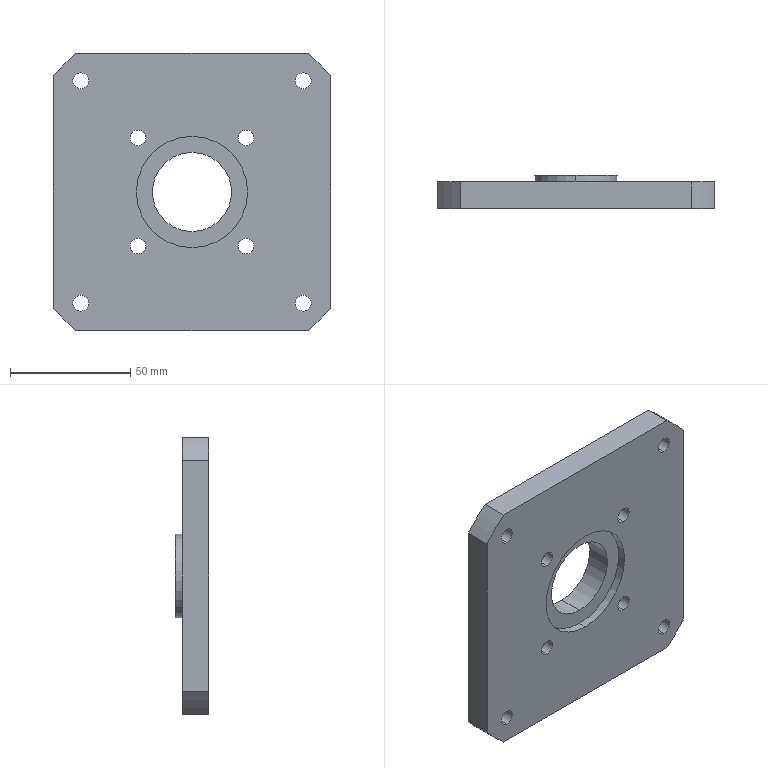Part | SolidWorks | features BaseBody 1 | 1 solid | 46 faces | box 115.385 x 13.846 x 115.385 mm | volume 127241 mm3 | cylinder 34 | plane 12 | commonest cylinder face diameters 6.577 x16 11.538 x8 150 x4 32.885 x2 34.615 x2 46.154 x2
STEP:
#1=CARTESIAN_POINT('',(184.809,206.,262.822));
#2=VERTEX_POINT('',#1);
#3=CARTESIAN_POINT('',(184.809,206.,274.36));
#4=VERTEX_POINT('',#3);
#5=CARTESIAN_POINT('',(184.809,206.,268.591));
#6=DIRECTION('',(0.,1.,0.));
#7=DIRECTION('',(0.,0.,1.));
#8=AXIS2_PLACEMENT_3D('',#5,#6,#7);
#9=CIRCLE('',#8,5.769);
#10=EDGE_CURVE('',#2,#4,#9,.T.);
#11=ORIENTED_EDGE('',*,*,#10,.F.);
#12=CARTESIAN_POINT('',(184.809,212.577,262.822));
#13=VERTEX_POINT('',#12);
#14=CARTESIAN_POINT('',(184.809,201.615,262.822));
#15=DIRECTION('',(0.,1.,0.));
#16=VECTOR('',#15,1000.);
#17=LINE('',#14,#16);
#18=EDGE_CURVE('',#2,#13,#17,.T.);
#19=ORIENTED_EDGE('',*,*,#18,.T.);
#20=CARTESIAN_POINT('',(184.809,212.577,274.36));
#21=VERTEX_POINT('',#20);
#22=CARTESIAN_POINT('',(184.809,212.577,268.591));
#23=DIRECTION('',(0.,1.,0.));
#24=DIRECTION('',(0.,0.,1.));
#25=AXIS2_PLACEMENT_3D('',#22,#23,#24);
#26=CIRCLE('',#25,5.769);
#27=EDGE_CURVE('',#13,#21,#26,.T.);
#28=ORIENTED_EDGE('',*,*,#27,.T.);
#29=CARTESIAN_POINT('',(184.809,201.615,274.36));
#30=DIRECTION('',(0.,1.,0.));
#31=VECTOR('',#30,1000.);
#32=LINE('',#29,#31);
#33=EDGE_CURVE('',#4,#21,#32,.T.);
#34=ORIENTED_EDGE('',*,*,#33,.F.);
#35=EDGE_LOOP('',(#11,#19,#28,#34));
#36=FACE_OUTER_BOUND('',#35,.T.);
#37=CARTESIAN_POINT('',(184.809,201.615,268.591));
#38=DIRECTION('',(0.,1.,0.));
#39=DIRECTION('',(0.,0.,1.));
#40=AXIS2_PLACEMENT_3D('',#37,#38,#39);
#41=CYLINDRICAL_SURFACE('',#40,5.769);
#42=ADVANCED_FACE('',(#36),#41,.F.);
#43=CARTESIAN_POINT('',(184.809,206.,217.948));
#44=VERTEX_POINT('',#43);
#45=CARTESIAN_POINT('',(184.809,206.,229.486));
#46=VERTEX_POINT('',#45);
#47=CARTESIAN_POINT('',(184.809,206.,223.717));
#48=DIRECTION('',(0.,1.,0.));
#49=DIRECTION('',(0.,0.,1.));
#50=AXIS2_PLACEMENT_3D('',#47,#48,#49);
#51=CIRCLE('',#50,5.769);
#52=EDGE_CURVE('',#44,#46,#51,.T.);
#53=ORIENTED_EDGE('',*,*,#52,.F.);
#54=CARTESIAN_POINT('',(184.809,212.577,217.948));
#55=VERTEX_POINT('',#54);
#56=CARTESIAN_POINT('',(184.809,201.615,217.948));
#57=DIRECTION('',(0.,1.,0.));
#58=VECTOR('',#57,1000.);
#59=LINE('',#56,#58);
#60=EDGE_CURVE('',#44,#55,#59,.T.);
#61=ORIENTED_EDGE('',*,*,#60,.T.);
#62=CARTESIAN_POINT('',(184.809,212.577,229.486));
#63=VERTEX_POINT('',#62);
#64=CARTESIAN_POINT('',(184.809,212.577,223.717));
#65=DIRECTION('',(0.,1.,0.));
#66=DIRECTION('',(0.,0.,1.));
#67=AXIS2_PLACEMENT_3D('',#64,#65,#66);
#68=CIRCLE('',#67,5.769);
#69=EDGE_CURVE('',#55,#63,#68,.T.);
#70=ORIENTED_EDGE('',*,*,#69,.T.);
#71=CARTESIAN_POINT('',(184.809,201.615,229.486));
#72=DIRECTION('',(0.,1.,0.));
#73=VECTOR('',#72,1000.);
#74=LINE('',#71,#73);
#75=EDGE_CURVE('',#46,#63,#74,.T.);
#76=ORIENTED_EDGE('',*,*,#75,.F.);
#77=EDGE_LOOP('',(#53,#61,#70,#76));
#78=FACE_OUTER_BOUND('',#77,.T.);
#79=CARTESIAN_POINT('',(184.809,201.615,223.717));
#80=DIRECTION('',(0.,1.,0.));
#81=DIRECTION('',(0.,0.,1.));
#82=AXIS2_PLACEMENT_3D('',#79,#80,#81);
#83=CYLINDRICAL_SURFACE('',#82,5.769);
#84=ADVANCED_FACE('',(#78),#83,.F.);
#85=CARTESIAN_POINT('',(161.093,212.577,289.019));
#86=VERTEX_POINT('',#85);
#87=CARTESIAN_POINT('',(161.093,212.577,295.596));
#88=VERTEX_POINT('',#87);
#89=CARTESIAN_POINT('',(161.093,212.577,292.308));
#90=DIRECTION('',(0.,1.,0.));
#91=DIRECTION('',(0.,0.,-1.));
#92=AXIS2_PLACEMENT_3D('',#89,#90,#91);
#93=CIRCLE('',#92,3.288);
#94=EDGE_CURVE('',#86,#88,#93,.T.);
#95=ORIENTED_EDGE('',*,*,#94,.T.);
#96=CARTESIAN_POINT('',(161.093,201.615,295.596));
#97=VERTEX_POINT('',#96);
#98=CARTESIAN_POINT('',(161.093,212.577,295.596));
#99=DIRECTION('',(0.,-1.,0.));
#100=VECTOR('',#99,1000.);
#101=LINE('',#98,#100);
#102=EDGE_CURVE('',#88,#97,#101,.T.);
#103=ORIENTED_EDGE('',*,*,#102,.T.);
#104=CARTESIAN_POINT('',(161.093,201.615,289.019));
#105=VERTEX_POINT('',#104);
#106=CARTESIAN_POINT('',(161.093,201.615,292.308));
#107=DIRECTION('',(0.,1.,0.));
#108=DIRECTION('',(0.,0.,-1.));
#109=AXIS2_PLACEMENT_3D('',#106,#107,#108);
#110=CIRCLE('',#109,3.288);
#111=EDGE_CURVE('',#105,#97,#110,.T.);
#112=ORIENTED_EDGE('',*,*,#111,.F.);
#113=CARTESIAN_POINT('',(161.093,212.577,289.019));
#114=DIRECTION('',(0.,-1.,0.));
#115=VECTOR('',#114,1000.);
#116=LINE('',#113,#115);
#117=EDGE_CURVE('',#86,#105,#116,.T.);
#118=ORIENTED_EDGE('',*,*,#117,.F.);
#119=EDGE_LOOP('',(#95,#103,#112,#118));
#120=FACE_OUTER_BOUND('',#119,.T.);
#121=CARTESIAN_POINT('',(161.093,212.577,292.308));
#122=DIRECTION('',(0.,-1.,0.));
#123=DIRECTION('',(0.,0.,-1.));
#124=AXIS2_PLACEMENT_3D('',#121,#122,#123);
#125=CYLINDRICAL_SURFACE('',#124,3.288);
#126=ADVANCED_FACE('',(#120),#125,.F.);
#127=CARTESIAN_POINT('',(253.4,212.577,196.712));
#128=VERTEX_POINT('',#127);
#129=CARTESIAN_POINT('',(253.4,212.577,203.288));
#130=VERTEX_POINT('',#129);
#131=CARTESIAN_POINT('',(253.4,212.577,200.));
#132=DIRECTION('',(0.,1.,0.));
#133=DIRECTION('',(0.,0.,-1.));
#134=AXIS2_PLACEMENT_3D('',#131,#132,#133);
#135=CIRCLE('',#134,3.288);
#136=EDGE_CURVE('',#128,#130,#135,.T.);
#137=ORIENTED_EDGE('',*,*,#136,.T.);
#138=CARTESIAN_POINT('',(253.4,201.615,203.288));
#139=VERTEX_POINT('',#138);
#140=CARTESIAN_POINT('',(253.4,212.577,203.288));
#141=DIRECTION('',(0.,-1.,0.));
#142=VECTOR('',#141,1000.);
#143=LINE('',#140,#142);
#144=EDGE_CURVE('',#130,#139,#143,.T.);
#145=ORIENTED_EDGE('',*,*,#144,.T.);
#146=CARTESIAN_POINT('',(253.4,201.615,196.712));
#147=VERTEX_POINT('',#146);
#148=CARTESIAN_POINT('',(253.4,201.615,200.));
#149=DIRECTION('',(0.,1.,0.));
#150=DIRECTION('',(0.,0.,-1.));
#151=AXIS2_PLACEMENT_3D('',#148,#149,#150);
#152=CIRCLE('',#151,3.288);
#153=EDGE_CURVE('',#147,#139,#152,.T.);
#154=ORIENTED_EDGE('',*,*,#153,.F.);
#155=CARTESIAN_POINT('',(253.4,212.577,196.712));
#156=DIRECTION('',(0.,-1.,0.));
#157=VECTOR('',#156,1000.);
#158=LINE('',#155,#157);
#159=EDGE_CURVE('',#128,#147,#158,.T.);
#160=ORIENTED_EDGE('',*,*,#159,.F.);
#161=EDGE_LOOP('',(#137,#145,#154,#160));
#162=FACE_OUTER_BOUND('',#161,.T.);
#163=CARTESIAN_POINT('',(253.4,212.577,200.));
#164=DIRECTION('',(0.,-1.,0.));
#165=DIRECTION('',(0.,0.,-1.));
#166=AXIS2_PLACEMENT_3D('',#163,#164,#165);
#167=CYLINDRICAL_SURFACE('',#166,3.288);
#168=ADVANCED_FACE('',(#162),#167,.F.);
#169=CARTESIAN_POINT('',(229.684,206.,217.948));
#170=VERTEX_POINT('',#169);
#171=CARTESIAN_POINT('',(229.684,206.,229.486));
#172=VERTEX_POINT('',#171);
#173=CARTESIAN_POINT('',(229.684,206.,223.717));
#174=DIRECTION('',(0.,1.,0.));
#175=DIRECTION('',(0.,0.,1.));
#176=AXIS2_PLACEMENT_3D('',#173,#174,#175);
#177=CIRCLE('',#176,5.769);
#178=EDGE_CURVE('',#170,#172,#177,.T.);
#179=ORIENTED_EDGE('',*,*,#178,.F.);
#180=CARTESIAN_POINT('',(229.684,212.577,217.948));
#181=VERTEX_POINT('',#180);
#182=CARTESIAN_POINT('',(229.684,201.615,217.948));
#183=DIRECTION('',(0.,1.,0.));
#184=VECTOR('',#183,1000.);
#185=LINE('',#182,#184);
#186=EDGE_CURVE('',#170,#181,#185,.T.);
#187=ORIENTED_EDGE('',*,*,#186,.T.);
#188=CARTESIAN_POINT('',(229.684,212.577,229.486));
#189=VERTEX_POINT('',#188);
#190=CARTESIAN_POINT('',(229.684,212.577,223.717));
#191=DIRECTION('',(0.,1.,0.));
#192=DIRECTION('',(0.,0.,1.));
#193=AXIS2_PLACEMENT_3D('',#190,#191,#192);
#194=CIRCLE('',#193,5.769);
#195=EDGE_CURVE('',#181,#189,#194,.T.);
#196=ORIENTED_EDGE('',*,*,#195,.T.);
#197=CARTESIAN_POINT('',(229.684,201.615,229.486));
#198=DIRECTION('',(0.,1.,0.));
#199=VECTOR('',#198,1000.);
#200=LINE('',#197,#199);
#201=EDGE_CURVE('',#172,#189,#200,.T.);
#202=ORIENTED_EDGE('',*,*,#201,.F.);
#203=EDGE_LOOP('',(#179,#187,#196,#202));
#204=FACE_OUTER_BOUND('',#203,.T.);
#205=CARTESIAN_POINT('',(229.684,201.615,223.717));
#206=DIRECTION('',(0.,1.,0.));
#207=DIRECTION('',(0.,0.,1.));
#208=AXIS2_PLACEMENT_3D('',#205,#206,#207);
#209=CYLINDRICAL_SURFACE('',#208,5.769);
#210=ADVANCED_FACE('',(#204),#209,.F.);
#211=CARTESIAN_POINT('',(161.093,212.577,196.712));
#212=VERTEX_POINT('',#211);
#213=CARTESIAN_POINT('',(161.093,212.577,203.288));
#214=VERTEX_POINT('',#213);
#215=CARTESIAN_POINT('',(161.093,212.577,200.));
#216=DIRECTION('',(0.,1.,0.));
#217=DIRECTION('',(0.,0.,-1.));
#218=AXIS2_PLACEMENT_3D('',#215,#216,#217);
#219=CIRCLE('',#218,3.288);
#220=EDGE_CURVE('',#212,#214,#219,.T.);
#221=ORIENTED_EDGE('',*,*,#220,.T.);
#222=CARTESIAN_POINT('',(161.093,201.615,203.288));
#223=VERTEX_POINT('',#222);
#224=CARTESIAN_POINT('',(161.093,212.577,203.288));
#225=DIRECTION('',(0.,-1.,0.));
#226=VECTOR('',#225,1000.);
#227=LINE('',#224,#226);
#228=EDGE_CURVE('',#214,#223,#227,.T.);
#229=ORIENTED_EDGE('',*,*,#228,.T.);
#230=CARTESIAN_POINT('',(161.093,201.615,196.712));
#231=VERTEX_POINT('',#230);
#232=CARTESIAN_POINT('',(161.093,201.615,200.));
#233=DIRECTION('',(0.,1.,0.));
#234=DIRECTION('',(0.,0.,-1.));
#235=AXIS2_PLACEMENT_3D('',#232,#233,#234);
#236=CIRCLE('',#235,3.288);
#237=EDGE_CURVE('',#231,#223,#236,.T.);
#238=ORIENTED_EDGE('',*,*,#237,.F.);
#239=CARTESIAN_POINT('',(161.093,212.577,196.712));
#240=DIRECTION('',(0.,-1.,0.));
#241=VECTOR('',#240,1000.);
#242=LINE('',#239,#241);
#243=EDGE_CURVE('',#212,#231,#242,.T.);
#244=ORIENTED_EDGE('',*,*,#243,.F.);
#245=EDGE_LOOP('',(#221,#229,#238,#244));
#246=FACE_OUTER_BOUND('',#245,.T.);
#247=CARTESIAN_POINT('',(161.093,212.577,200.));
#248=DIRECTION('',(0.,-1.,0.));
#249=DIRECTION('',(0.,0.,-1.));
#250=AXIS2_PLACEMENT_3D('',#247,#248,#249);
#251=CYLINDRICAL_SURFACE('',#250,3.288);
#252=ADVANCED_FACE('',(#246),#251,.F.);
#253=CARTESIAN_POINT('',(253.4,212.577,289.019));
#254=VERTEX_POINT('',#253);
#255=CARTESIAN_POINT('',(253.4,212.577,295.596));
#256=VERTEX_POINT('',#255);
#257=CARTESIAN_POINT('',(253.4,212.577,292.308));
#258=DIRECTION('',(0.,1.,0.));
#259=DIRECTION('',(0.,0.,-1.));
#260=AXIS2_PLACEMENT_3D('',#257,#258,#259);
#261=CIRCLE('',#260,3.288);
#262=EDGE_CURVE('',#254,#256,#261,.T.);
#263=ORIENTED_EDGE('',*,*,#262,.T.);
#264=CARTESIAN_POINT('',(253.4,201.615,295.596));
#265=VERTEX_POINT('',#264);
#266=CARTESIAN_POINT('',(253.4,212.577,295.596));
#267=DIRECTION('',(0.,-1.,0.));
#268=VECTOR('',#267,1000.);
#269=LINE('',#266,#268);
#270=EDGE_CURVE('',#256,#265,#269,.T.);
#271=ORIENTED_EDGE('',*,*,#270,.T.);
#272=CARTESIAN_POINT('',(253.4,201.615,289.019));
#273=VERTEX_POINT('',#272);
#274=CARTESIAN_POINT('',(253.4,201.615,292.308));
#275=DIRECTION('',(0.,1.,0.));
#276=DIRECTION('',(0.,0.,-1.));
#277=AXIS2_PLACEMENT_3D('',#274,#275,#276);
#278=CIRCLE('',#277,3.288);
#279=EDGE_CURVE('',#273,#265,#278,.T.);
#280=ORIENTED_EDGE('',*,*,#279,.F.);
#281=CARTESIAN_POINT('',(253.4,212.577,289.019));
#282=DIRECTION('',(0.,-1.,0.));
#283=VECTOR('',#282,1000.);
#284=LINE('',#281,#283);
#285=EDGE_CURVE('',#254,#273,#284,.T.);
#286=ORIENTED_EDGE('',*,*,#285,.F.);
#287=EDGE_LOOP('',(#263,#271,#280,#286));
#288=FACE_OUTER_BOUND('',#287,.T.);
#289=CARTESIAN_POINT('',(253.4,212.577,292.308));
#290=DIRECTION('',(0.,-1.,0.));
#291=DIRECTION('',(0.,0.,-1.));
#292=AXIS2_PLACEMENT_3D('',#289,#290,#291);
#293=CYLINDRICAL_SURFACE('',#292,3.288);
#294=ADVANCED_FACE('',(#288),#293,.F.);
#295=CARTESIAN_POINT('',(207.247,215.462,228.846));
#296=VERTEX_POINT('',#295);
#297=CARTESIAN_POINT('',(207.247,215.462,263.462));
#298=VERTEX_POINT('',#297);
#299=CARTESIAN_POINT('',(207.247,215.462,246.154));
#300=DIRECTION('',(0.,-1.,0.));
#301=DIRECTION('',(0.,0.,-1.));
#302=AXIS2_PLACEMENT_3D('',#299,#300,#301);
#303=CIRCLE('',#302,17.308);
#304=EDGE_CURVE('',#296,#298,#303,.T.);
#305=ORIENTED_EDGE('',*,*,#304,.T.);
#306=CARTESIAN_POINT('',(207.247,212.577,263.462));
#307=VERTEX_POINT('',#306);
#308=CARTESIAN_POINT('',(207.247,215.462,263.462));
#309=DIRECTION('',(0.,-1.,0.));
#310=VECTOR('',#309,1000.);
#311=LINE('',#308,#310);
#312=EDGE_CURVE('',#298,#307,#311,.T.);
#313=ORIENTED_EDGE('',*,*,#312,.T.);
#314=CARTESIAN_POINT('',(207.247,212.577,228.846));
#315=VERTEX_POINT('',#314);
#316=CARTESIAN_POINT('',(207.247,212.577,246.154));
#317=DIRECTION('',(0.,1.,0.));
#318=DIRECTION('',(0.,0.,-1.));
#319=AXIS2_PLACEMENT_3D('',#316,#317,#318);
#320=CIRCLE('',#319,17.308);
#321=EDGE_CURVE('',#307,#315,#320,.T.);
#322=ORIENTED_EDGE('',*,*,#321,.T.);
#323=CARTESIAN_POINT('',(207.247,215.462,228.846));
#324=DIRECTION('',(0.,-1.,0.));
#325=VECTOR('',#324,1000.);
#326=LINE('',#323,#325);
#327=EDGE_CURVE('',#296,#315,#326,.T.);
#328=ORIENTED_EDGE('',*,*,#327,.F.);
#329=EDGE_LOOP('',(#305,#313,#322,#328));
#330=FACE_OUTER_BOUND('',#329,.T.);
#331=CARTESIAN_POINT('',(207.247,215.462,246.154));
#332=DIRECTION('',(0.,-1.,0.));
#333=DIRECTION('',(0.,0.,-1.));
#334=AXIS2_PLACEMENT_3D('',#331,#332,#333);
#335=CYLINDRICAL_SURFACE('',#334,17.308);
#336=ADVANCED_FACE('',(#330),#335,.T.);
#337=CARTESIAN_POINT('',(229.684,206.,262.822));
#338=VERTEX_POINT('',#337);
#339=CARTESIAN_POINT('',(229.684,206.,274.36));
#340=VERTEX_POINT('',#339);
#341=CARTESIAN_POINT('',(229.684,206.,268.591));
#342=DIRECTION('',(0.,1.,0.));
#343=DIRECTION('',(0.,0.,1.));
#344=AXIS2_PLACEMENT_3D('',#341,#342,#343);
#345=CIRCLE('',#344,5.769);
#346=EDGE_CURVE('',#338,#340,#345,.T.);
#347=ORIENTED_EDGE('',*,*,#346,.F.);
#348=CARTESIAN_POINT('',(229.684,212.577,262.822));
#349=VERTEX_POINT('',#348);
#350=CARTESIAN_POINT('',(229.684,201.615,262.822));
#351=DIRECTION('',(0.,1.,0.));
#352=VECTOR('',#351,1000.);
#353=LINE('',#350,#352);
#354=EDGE_CURVE('',#338,#349,#353,.T.);
#355=ORIENTED_EDGE('',*,*,#354,.T.);
#356=CARTESIAN_POINT('',(229.684,212.577,274.36));
#357=VERTEX_POINT('',#356);
#358=CARTESIAN_POINT('',(229.684,212.577,268.591));
#359=DIRECTION('',(0.,1.,0.));
#360=DIRECTION('',(0.,0.,1.));
#361=AXIS2_PLACEMENT_3D('',#358,#359,#360);
#362=CIRCLE('',#361,5.769);
#363=EDGE_CURVE('',#349,#357,#362,.T.);
#364=ORIENTED_EDGE('',*,*,#363,.T.);
#365=CARTESIAN_POINT('',(229.684,201.615,274.36));
#366=DIRECTION('',(0.,1.,0.));
#367=VECTOR('',#366,1000.);
#368=LINE('',#365,#367);
#369=EDGE_CURVE('',#340,#357,#368,.T.);
#370=ORIENTED_EDGE('',*,*,#369,.F.);
#371=EDGE_LOOP('',(#347,#355,#364,#370));
#372=FACE_OUTER_BOUND('',#371,.T.);
#373=CARTESIAN_POINT('',(229.684,201.615,268.591));
#374=DIRECTION('',(0.,1.,0.));
#375=DIRECTION('',(0.,0.,1.));
#376=AXIS2_PLACEMENT_3D('',#373,#374,#375);
#377=CYLINDRICAL_SURFACE('',#376,5.769);
#378=ADVANCED_FACE('',(#372),#377,.F.);
#379=CARTESIAN_POINT('',(184.809,201.615,265.302));
#380=VERTEX_POINT('',#379);
#381=CARTESIAN_POINT('',(184.809,201.615,271.879));
#382=VERTEX_POINT('',#381);
#383=CARTESIAN_POINT('',(184.809,201.615,268.591));
#384=DIRECTION('',(0.,1.,0.));
#385=DIRECTION('',(0.,0.,1.));
#386=AXIS2_PLACEMENT_3D('',#383,#384,#385);
#387=CIRCLE('',#386,3.288);
#388=EDGE_CURVE('',#380,#382,#387,.T.);
#389=ORIENTED_EDGE('',*,*,#388,.F.);
#390=CARTESIAN_POINT('',(184.809,206.,265.302));
#391=VERTEX_POINT('',#390);
#392=CARTESIAN_POINT('',(184.809,201.615,265.302));
#393=DIRECTION('',(0.,1.,0.));
#394=VECTOR('',#393,1000.);
#395=LINE('',#392,#394);
#396=EDGE_CURVE('',#380,#391,#395,.T.);
#397=ORIENTED_EDGE('',*,*,#396,.T.);
#398=CARTESIAN_POINT('',(184.809,206.,271.879));
#399=VERTEX_POINT('',#398);
#400=CARTESIAN_POINT('',(184.809,206.,268.591));
#401=DIRECTION('',(0.,-1.,0.));
#402=DIRECTION('',(0.,0.,1.));
#403=AXIS2_PLACEMENT_3D('',#400,#401,#402);
#404=CIRCLE('',#403,3.288);
#405=EDGE_CURVE('',#399,#391,#404,.T.);
#406=ORIENTED_EDGE('',*,*,#405,.F.);
#407=CARTESIAN_POINT('',(184.809,201.615,271.879));
#408=DIRECTION('',(0.,1.,0.));
#409=VECTOR('',#408,1000.);
#410=LINE('',#407,#409);
#411=EDGE_CURVE('',#382,#399,#410,.T.);
#412=ORIENTED_EDGE('',*,*,#411,.F.);
#413=EDGE_LOOP('',(#389,#397,#406,#412));
#414=FACE_OUTER_BOUND('',#413,.T.);
#415=CARTESIAN_POINT('',(184.809,201.615,268.591));
#416=DIRECTION('',(0.,1.,0.));
#417=DIRECTION('',(0.,0.,1.));
#418=AXIS2_PLACEMENT_3D('',#415,#416,#417);
#419=CYLINDRICAL_SURFACE('',#418,3.288);
#420=ADVANCED_FACE('',(#414),#419,.F.);
#421=CARTESIAN_POINT('',(184.809,201.615,220.428));
#422=VERTEX_POINT('',#421);
#423=CARTESIAN_POINT('',(184.809,201.615,227.005));
#424=VERTEX_POINT('',#423);
#425=CARTESIAN_POINT('',(184.809,201.615,223.717));
#426=DIRECTION('',(0.,1.,0.));
#427=DIRECTION('',(0.,0.,1.));
#428=AXIS2_PLACEMENT_3D('',#425,#426,#427);
#429=CIRCLE('',#428,3.288);
#430=EDGE_CURVE('',#422,#424,#429,.T.);
#431=ORIENTED_EDGE('',*,*,#430,.F.);
#432=CARTESIAN_POINT('',(184.809,206.,220.428));
#433=VERTEX_POINT('',#432);
#434=CARTESIAN_POINT('',(184.809,201.615,220.428));
#435=DIRECTION('',(0.,1.,0.));
#436=VECTOR('',#435,1000.);
#437=LINE('',#434,#436);
#438=EDGE_CURVE('',#422,#433,#437,.T.);
#439=ORIENTED_EDGE('',*,*,#438,.T.);
#440=CARTESIAN_POINT('',(184.809,206.,227.005));
#441=VERTEX_POINT('',#440);
#442=CARTESIAN_POINT('',(184.809,206.,223.717));
#443=DIRECTION('',(0.,-1.,0.));
#444=DIRECTION('',(0.,0.,1.));
#445=AXIS2_PLACEMENT_3D('',#442,#443,#444);
#446=CIRCLE('',#445,3.288);
#447=EDGE_CURVE('',#441,#433,#446,.T.);
#448=ORIENTED_EDGE('',*,*,#447,.F.);
#449=CARTESIAN_POINT('',(184.809,201.615,227.005));
#450=DIRECTION('',(0.,1.,0.));
#451=VECTOR('',#450,1000.);
#452=LINE('',#449,#451);
#453=EDGE_CURVE('',#424,#441,#452,.T.);
#454=ORIENTED_EDGE('',*,*,#453,.F.);
#455=EDGE_LOOP('',(#431,#439,#448,#454));
#456=FACE_OUTER_BOUND('',#455,.T.);
#457=CARTESIAN_POINT('',(184.809,201.615,223.717));
#458=DIRECTION('',(0.,1.,0.));
#459=DIRECTION('',(0.,0.,1.));
#460=AXIS2_PLACEMENT_3D('',#457,#458,#459);
#461=CYLINDRICAL_SURFACE('',#460,3.288);
#462=ADVANCED_FACE('',(#456),#461,.F.);
#463=CARTESIAN_POINT('',(229.684,201.615,220.428));
#464=VERTEX_POINT('',#463);
#465=CARTESIAN_POINT('',(229.684,201.615,227.005));
#466=VERTEX_POINT('',#465);
#467=CARTESIAN_POINT('',(229.684,201.615,223.717));
#468=DIRECTION('',(0.,1.,0.));
#469=DIRECTION('',(0.,0.,1.));
#470=AXIS2_PLACEMENT_3D('',#467,#468,#469);
#471=CIRCLE('',#470,3.288);
#472=EDGE_CURVE('',#464,#466,#471,.T.);
#473=ORIENTED_EDGE('',*,*,#472,.F.);
#474=CARTESIAN_POINT('',(229.684,206.,220.428));
#475=VERTEX_POINT('',#474);
#476=CARTESIAN_POINT('',(229.684,201.615,220.428));
#477=DIRECTION('',(0.,1.,0.));
#478=VECTOR('',#477,1000.);
#479=LINE('',#476,#478);
#480=EDGE_CURVE('',#464,#475,#479,.T.);
#481=ORIENTED_EDGE('',*,*,#480,.T.);
#482=CARTESIAN_POINT('',(229.684,206.,227.005));
#483=VERTEX_POINT('',#482);
#484=CARTESIAN_POINT('',(229.684,206.,223.717));
#485=DIRECTION('',(0.,-1.,0.));
#486=DIRECTION('',(0.,0.,1.));
#487=AXIS2_PLACEMENT_3D('',#484,#485,#486);
#488=CIRCLE('',#487,3.288);
#489=EDGE_CURVE('',#483,#475,#488,.T.);
#490=ORIENTED_EDGE('',*,*,#489,.F.);
#491=CARTESIAN_POINT('',(229.684,201.615,227.005));
#492=DIRECTION('',(0.,1.,0.));
#493=VECTOR('',#492,1000.);
#494=LINE('',#491,#493);
#495=EDGE_CURVE('',#466,#483,#494,.T.);
#496=ORIENTED_EDGE('',*,*,#495,.F.);
#497=EDGE_LOOP('',(#473,#481,#490,#496));
#498=FACE_OUTER_BOUND('',#497,.T.);
#499=CARTESIAN_POINT('',(229.684,201.615,223.717));
#500=DIRECTION('',(0.,1.,0.));
#501=DIRECTION('',(0.,0.,1.));
#502=AXIS2_PLACEMENT_3D('',#499,#500,#501);
#503=CYLINDRICAL_SURFACE('',#502,3.288);
#504=ADVANCED_FACE('',(#498),#503,.F.);
#505=CARTESIAN_POINT('',(207.247,205.077,269.231));
#506=VERTEX_POINT('',#505);
#507=CARTESIAN_POINT('',(207.247,205.077,223.077));
#508=VERTEX_POINT('',#507);
#509=CARTESIAN_POINT('',(207.247,205.077,246.154));
#510=DIRECTION('',(0.,-1.,0.));
#511=DIRECTION('',(0.,0.,-1.));
#512=AXIS2_PLACEMENT_3D('',#509,#510,#511);
#513=CIRCLE('',#512,23.077);
#514=EDGE_CURVE('',#506,#508,#513,.T.);
#515=ORIENTED_EDGE('',*,*,#514,.F.);
#516=CARTESIAN_POINT('',(207.247,201.615,269.231));
#517=VERTEX_POINT('',#516);
#518=CARTESIAN_POINT('',(207.247,215.462,269.231));
#519=DIRECTION('',(0.,-1.,0.));
#520=VECTOR('',#519,1000.);
#521=LINE('',#518,#520);
#522=EDGE_CURVE('',#506,#517,#521,.T.);
#523=ORIENTED_EDGE('',*,*,#522,.T.);
#524=CARTESIAN_POINT('',(207.247,201.615,223.077));
#525=VERTEX_POINT('',#524);
#526=CARTESIAN_POINT('',(207.247,201.615,246.154));
#527=DIRECTION('',(0.,1.,0.));
#528=DIRECTION('',(0.,0.,-1.));
#529=AXIS2_PLACEMENT_3D('',#526,#527,#528);
#530=CIRCLE('',#529,23.077);
#531=EDGE_CURVE('',#525,#517,#530,.T.);
#532=ORIENTED_EDGE('',*,*,#531,.F.);
#533=CARTESIAN_POINT('',(207.247,215.462,223.077));
#534=DIRECTION('',(0.,-1.,0.));
#535=VECTOR('',#534,1000.);
#536=LINE('',#533,#535);
#537=EDGE_CURVE('',#508,#525,#536,.T.);
#538=ORIENTED_EDGE('',*,*,#537,.F.);
#539=EDGE_LOOP('',(#515,#523,#532,#538));
#540=FACE_OUTER_BOUND('',#539,.T.);
#541=CARTESIAN_POINT('',(207.247,215.462,246.154));
#542=DIRECTION('',(0.,-1.,0.));
#543=DIRECTION('',(0.,0.,-1.));
#544=AXIS2_PLACEMENT_3D('',#541,#542,#543);
#545=CYLINDRICAL_SURFACE('',#544,23.077);
#546=ADVANCED_FACE('',(#540),#545,.F.);
#547=CARTESIAN_POINT('',(229.684,201.615,265.302));
#548=VERTEX_POINT('',#547);
#549=CARTESIAN_POINT('',(229.684,201.615,271.879));
#550=VERTEX_POINT('',#549);
#551=CARTESIAN_POINT('',(229.684,201.615,268.591));
#552=DIRECTION('',(0.,1.,0.));
#553=DIRECTION('',(0.,0.,1.));
#554=AXIS2_PLACEMENT_3D('',#551,#552,#553);
#555=CIRCLE('',#554,3.288);
#556=EDGE_CURVE('',#548,#550,#555,.T.);
#557=ORIENTED_EDGE('',*,*,#556,.F.);
#558=CARTESIAN_POINT('',(229.684,206.,265.302));
#559=VERTEX_POINT('',#558);
#560=CARTESIAN_POINT('',(229.684,201.615,265.302));
#561=DIRECTION('',(0.,1.,0.));
#562=VECTOR('',#561,1000.);
#563=LINE('',#560,#562);
#564=EDGE_CURVE('',#548,#559,#563,.T.);
#565=ORIENTED_EDGE('',*,*,#564,.T.);
#566=CARTESIAN_POINT('',(229.684,206.,271.879));
#567=VERTEX_POINT('',#566);
#568=CARTESIAN_POINT('',(229.684,206.,268.591));
#569=DIRECTION('',(0.,-1.,0.));
#570=DIRECTION('',(0.,0.,1.));
#571=AXIS2_PLACEMENT_3D('',#568,#569,#570);
#572=CIRCLE('',#571,3.288);
#573=EDGE_CURVE('',#567,#559,#572,.T.);
#574=ORIENTED_EDGE('',*,*,#573,.F.);
#575=CARTESIAN_POINT('',(229.684,201.615,271.879));
#576=DIRECTION('',(0.,1.,0.));
#577=VECTOR('',#576,1000.);
#578=LINE('',#575,#577);
#579=EDGE_CURVE('',#550,#567,#578,.T.);
#580=ORIENTED_EDGE('',*,*,#579,.F.);
#581=EDGE_LOOP('',(#557,#565,#574,#580));
#582=FACE_OUTER_BOUND('',#581,.T.);
#583=CARTESIAN_POINT('',(229.684,201.615,268.591));
#584=DIRECTION('',(0.,1.,0.));
#585=DIRECTION('',(0.,0.,1.));
#586=AXIS2_PLACEMENT_3D('',#583,#584,#585);
#587=CYLINDRICAL_SURFACE('',#586,3.288);
#588=ADVANCED_FACE('',(#582),#587,.F.);
#589=CARTESIAN_POINT('',(207.247,215.462,229.712));
#590=VERTEX_POINT('',#589);
#591=CARTESIAN_POINT('',(207.247,215.462,262.596));
#592=VERTEX_POINT('',#591);
#593=CARTESIAN_POINT('',(207.247,215.462,246.154));
#594=DIRECTION('',(0.,1.,0.));
#595=DIRECTION('',(0.,0.,-1.));
#596=AXIS2_PLACEMENT_3D('',#593,#594,#595);
#597=CIRCLE('',#596,16.442);
#598=EDGE_CURVE('',#590,#592,#597,.T.);
#599=ORIENTED_EDGE('',*,*,#598,.T.);
#600=CARTESIAN_POINT('',(207.247,205.077,262.596));
#601=VERTEX_POINT('',#600);
#602=CARTESIAN_POINT('',(207.247,215.462,262.596));
#603=DIRECTION('',(0.,-1.,0.));
#604=VECTOR('',#603,1000.);
#605=LINE('',#602,#604);
#606=EDGE_CURVE('',#592,#601,#605,.T.);
#607=ORIENTED_EDGE('',*,*,#606,.T.);
#608=CARTESIAN_POINT('',(207.247,205.077,229.712));
#609=VERTEX_POINT('',#608);
#610=CARTESIAN_POINT('',(207.247,205.077,246.154));
#611=DIRECTION('',(0.,1.,0.));
#612=DIRECTION('',(0.,0.,-1.));
#613=AXIS2_PLACEMENT_3D('',#610,#611,#612);
#614=CIRCLE('',#613,16.442);
#615=EDGE_CURVE('',#609,#601,#614,.T.);
#616=ORIENTED_EDGE('',*,*,#615,.F.);
#617=CARTESIAN_POINT('',(207.247,215.462,229.712));
#618=DIRECTION('',(0.,-1.,0.));
#619=VECTOR('',#618,1000.);
#620=LINE('',#617,#619);
#621=EDGE_CURVE('',#590,#609,#620,.T.);
#622=ORIENTED_EDGE('',*,*,#621,.F.);
#623=EDGE_LOOP('',(#599,#607,#616,#622));
#624=FACE_OUTER_BOUND('',#623,.T.);
#625=CARTESIAN_POINT('',(207.247,215.462,246.154));
#626=DIRECTION('',(0.,-1.,0.));
#627=DIRECTION('',(0.,0.,-1.));
#628=AXIS2_PLACEMENT_3D('',#625,#626,#627);
#629=CYLINDRICAL_SURFACE('',#628,16.442);
#630=ADVANCED_FACE('',(#624),#629,.F.);
#631=CARTESIAN_POINT('',(184.809,212.577,268.591));
#632=DIRECTION('',(0.,1.,0.));
#633=DIRECTION('',(0.,0.,1.));
#634=AXIS2_PLACEMENT_3D('',#631,#632,#633);
#635=CIRCLE('',#634,5.769);
#636=EDGE_CURVE('',#21,#13,#635,.T.);
#637=ORIENTED_EDGE('',*,*,#636,.F.);
#638=ORIENTED_EDGE('',*,*,#27,.F.);
#639=EDGE_LOOP('',(#637,#638));
#640=FACE_BOUND('',#639,.T.);
#641=CARTESIAN_POINT('',(184.809,212.577,223.717));
#642=DIRECTION('',(0.,1.,0.));
#643=DIRECTION('',(0.,0.,1.));
#644=AXIS2_PLACEMENT_3D('',#641,#642,#643);
#645=CIRCLE('',#644,5.769);
#646=EDGE_CURVE('',#63,#55,#645,.T.);
#647=ORIENTED_EDGE('',*,*,#646,.F.);
#648=ORIENTED_EDGE('',*,*,#69,.F.);
#649=EDGE_LOOP('',(#647,#648));
#650=FACE_BOUND('',#649,.T.);
#651=ORIENTED_EDGE('',*,*,#94,.F.);
#652=CARTESIAN_POINT('',(161.093,212.577,292.308));
#653=DIRECTION('',(0.,1.,0.));
#654=DIRECTION('',(0.,0.,-1.));
#655=AXIS2_PLACEMENT_3D('',#652,#653,#654);
#656=CIRCLE('',#655,3.288);
#657=EDGE_CURVE('',#88,#86,#656,.T.);
#658=ORIENTED_EDGE('',*,*,#657,.F.);
#659=EDGE_LOOP('',(#651,#658));
#660=FACE_BOUND('',#659,.T.);
#661=ORIENTED_EDGE('',*,*,#136,.F.);
#662=CARTESIAN_POINT('',(253.4,212.577,200.));
#663=DIRECTION('',(0.,1.,0.));
#664=DIRECTION('',(0.,0.,-1.));
#665=AXIS2_PLACEMENT_3D('',#662,#663,#664);
#666=CIRCLE('',#665,3.288);
#667=EDGE_CURVE('',#130,#128,#666,.T.);
#668=ORIENTED_EDGE('',*,*,#667,.F.);
#669=EDGE_LOOP('',(#661,#668));
#670=FACE_BOUND('',#669,.T.);
#671=CARTESIAN_POINT('',(229.684,212.577,223.717));
#672=DIRECTION('',(0.,1.,0.));
#673=DIRECTION('',(0.,0.,1.));
#674=AXIS2_PLACEMENT_3D('',#671,#672,#673);
#675=CIRCLE('',#674,5.769);
#676=EDGE_CURVE('',#189,#181,#675,.T.);
#677=ORIENTED_EDGE('',*,*,#676,.F.);
#678=ORIENTED_EDGE('',*,*,#195,.F.);
#679=EDGE_LOOP('',(#677,#678));
#680=FACE_BOUND('',#679,.T.);
#681=ORIENTED_EDGE('',*,*,#220,.F.);
#682=CARTESIAN_POINT('',(161.093,212.577,200.));
#683=DIRECTION('',(0.,1.,0.));
#684=DIRECTION('',(0.,0.,-1.));
#685=AXIS2_PLACEMENT_3D('',#682,#683,#684);
#686=CIRCLE('',#685,3.288);
#687=EDGE_CURVE('',#214,#212,#686,.T.);
#688=ORIENTED_EDGE('',*,*,#687,.F.);
#689=EDGE_LOOP('',(#681,#688));
#690=FACE_BOUND('',#689,.T.);
#691=ORIENTED_EDGE('',*,*,#262,.F.);
#692=CARTESIAN_POINT('',(253.4,212.577,292.308));
#693=DIRECTION('',(0.,1.,0.));
#694=DIRECTION('',(0.,0.,-1.));
#695=AXIS2_PLACEMENT_3D('',#692,#693,#694);
#696=CIRCLE('',#695,3.288);
#697=EDGE_CURVE('',#256,#254,#696,.T.);
#698=ORIENTED_EDGE('',*,*,#697,.F.);
#699=EDGE_LOOP('',(#691,#698));
#700=FACE_BOUND('',#699,.T.);
#701=CARTESIAN_POINT('',(207.247,212.577,246.154));
#702=DIRECTION('',(0.,1.,0.));
#703=DIRECTION('',(0.,0.,-1.));
#704=AXIS2_PLACEMENT_3D('',#701,#702,#703);
#705=CIRCLE('',#704,17.308);
#706=EDGE_CURVE('',#315,#307,#705,.T.);
#707=ORIENTED_EDGE('',*,*,#706,.F.);
#708=ORIENTED_EDGE('',*,*,#321,.F.);
#709=EDGE_LOOP('',(#707,#708));
#710=FACE_BOUND('',#709,.T.);
#711=CARTESIAN_POINT('',(229.684,212.577,268.591));
#712=DIRECTION('',(0.,1.,0.));
#713=DIRECTION('',(0.,0.,1.));
#714=AXIS2_PLACEMENT_3D('',#711,#712,#713);
#715=CIRCLE('',#714,5.769);
#716=EDGE_CURVE('',#357,#349,#715,.T.);
#717=ORIENTED_EDGE('',*,*,#716,.F.);
#718=ORIENTED_EDGE('',*,*,#363,.F.);
#719=EDGE_LOOP('',(#717,#718));
#720=FACE_BOUND('',#719,.T.);
#721=CARTESIAN_POINT('',(149.554,212.577,198.231));
#722=VERTEX_POINT('',#721);
#723=CARTESIAN_POINT('',(159.324,212.577,188.462));
#724=VERTEX_POINT('',#723);
#725=CARTESIAN_POINT('',(207.247,212.577,246.154));
#726=DIRECTION('',(0.,-1.,0.));
#727=DIRECTION('',(0.,0.,-1.));
#728=AXIS2_PLACEMENT_3D('',#725,#726,#727);
#729=CIRCLE('',#728,75.);
#730=EDGE_CURVE('',#722,#724,#729,.T.);
#731=ORIENTED_EDGE('',*,*,#730,.F.);
#732=CARTESIAN_POINT('',(149.554,212.577,294.077));
#733=VERTEX_POINT('',#732);
#734=CARTESIAN_POINT('',(149.554,212.577,246.154));
#735=DIRECTION('',(0.,0.,-1.));
#736=VECTOR('',#735,1000.);
#737=LINE('',#734,#736);
#738=EDGE_CURVE('',#733,#722,#737,.T.);
#739=ORIENTED_EDGE('',*,*,#738,.F.);
#740=CARTESIAN_POINT('',(159.324,212.577,303.846));
#741=VERTEX_POINT('',#740);
#742=CARTESIAN_POINT('',(207.247,212.577,246.154));
#743=DIRECTION('',(0.,-1.,0.));
#744=DIRECTION('',(0.,0.,-1.));
#745=AXIS2_PLACEMENT_3D('',#742,#743,#744);
#746=CIRCLE('',#745,75.);
#747=EDGE_CURVE('',#741,#733,#746,.T.);
#748=ORIENTED_EDGE('',*,*,#747,.F.);
#749=CARTESIAN_POINT('',(255.169,212.577,303.846));
#750=VERTEX_POINT('',#749);
#751=CARTESIAN_POINT('',(207.247,212.577,303.846));
#752=DIRECTION('',(-1.,0.,0.));
#753=VECTOR('',#752,1000.);
#754=LINE('',#751,#753);
#755=EDGE_CURVE('',#750,#741,#754,.T.);
#756=ORIENTED_EDGE('',*,*,#755,.F.);
#757=CARTESIAN_POINT('',(264.939,212.577,294.077));
#758=VERTEX_POINT('',#757);
#759=CARTESIAN_POINT('',(207.247,212.577,246.154));
#760=DIRECTION('',(0.,-1.,0.));
#761=DIRECTION('',(0.,0.,-1.));
#762=AXIS2_PLACEMENT_3D('',#759,#760,#761);
#763=CIRCLE('',#762,75.);
#764=EDGE_CURVE('',#758,#750,#763,.T.);
#765=ORIENTED_EDGE('',*,*,#764,.F.);
#766=CARTESIAN_POINT('',(264.939,212.577,198.231));
#767=VERTEX_POINT('',#766);
#768=CARTESIAN_POINT('',(264.939,212.577,246.154));
#769=DIRECTION('',(0.,0.,1.));
#770=VECTOR('',#769,1000.);
#771=LINE('',#768,#770);
#772=EDGE_CURVE('',#767,#758,#771,.T.);
#773=ORIENTED_EDGE('',*,*,#772,.F.);
#774=CARTESIAN_POINT('',(255.169,212.577,188.462));
#775=VERTEX_POINT('',#774);
#776=CARTESIAN_POINT('',(207.247,212.577,246.154));
#777=DIRECTION('',(0.,-1.,0.));
#778=DIRECTION('',(0.,0.,-1.));
#779=AXIS2_PLACEMENT_3D('',#776,#777,#778);
#780=CIRCLE('',#779,75.);
#781=EDGE_CURVE('',#775,#767,#780,.T.);
#782=ORIENTED_EDGE('',*,*,#781,.F.);
#783=CARTESIAN_POINT('',(207.247,212.577,188.462));
#784=DIRECTION('',(1.,0.,0.));
#785=VECTOR('',#784,1000.);
#786=LINE('',#783,#785);
#787=EDGE_CURVE('',#724,#775,#786,.T.);
#788=ORIENTED_EDGE('',*,*,#787,.F.);
#789=EDGE_LOOP('',(#731,#739,#748,#756,#765,#773,#782,#788));
#790=FACE_OUTER_BOUND('',#789,.T.);
#791=CARTESIAN_POINT('',(207.247,212.577,246.154));
#792=DIRECTION('',(0.,-1.,0.));
#793=DIRECTION('',(0.,0.,-1.));
#794=AXIS2_PLACEMENT_3D('',#791,#792,#793);
#795=PLANE('',#794);
#796=ADVANCED_FACE('',(#640,#650,#660,#670,#680,#690,#700,#710,#720,#790),#795,.F.);
#797=ORIENTED_EDGE('',*,*,#18,.F.);
#798=CARTESIAN_POINT('',(184.809,206.,268.591));
#799=DIRECTION('',(0.,1.,0.));
#800=DIRECTION('',(0.,0.,1.));
#801=AXIS2_PLACEMENT_3D('',#798,#799,#800);
#802=CIRCLE('',#801,5.769);
#803=EDGE_CURVE('',#4,#2,#802,.T.);
#804=ORIENTED_EDGE('',*,*,#803,.F.);
#805=ORIENTED_EDGE('',*,*,#33,.T.);
#806=ORIENTED_EDGE('',*,*,#636,.T.);
#807=EDGE_LOOP('',(#797,#804,#805,#806));
#808=FACE_OUTER_BOUND('',#807,.T.);
#809=CARTESIAN_POINT('',(184.809,201.615,268.591));
#810=DIRECTION('',(0.,1.,0.));
#811=DIRECTION('',(0.,0.,1.));
#812=AXIS2_PLACEMENT_3D('',#809,#810,#811);
#813=CYLINDRICAL_SURFACE('',#812,5.769);
#814=ADVANCED_FACE('',(#808),#813,.F.);
#815=ORIENTED_EDGE('',*,*,#60,.F.);
#816=CARTESIAN_POINT('',(184.809,206.,223.717));
#817=DIRECTION('',(0.,1.,0.));
#818=DIRECTION('',(0.,0.,1.));
#819=AXIS2_PLACEMENT_3D('',#816,#817,#818);
#820=CIRCLE('',#819,5.769);
#821=EDGE_CURVE('',#46,#44,#820,.T.);
#822=ORIENTED_EDGE('',*,*,#821,.F.);
#823=ORIENTED_EDGE('',*,*,#75,.T.);
#824=ORIENTED_EDGE('',*,*,#646,.T.);
#825=EDGE_LOOP('',(#815,#822,#823,#824));
#826=FACE_OUTER_BOUND('',#825,.T.);
#827=CARTESIAN_POINT('',(184.809,201.615,223.717));
#828=DIRECTION('',(0.,1.,0.));
#829=DIRECTION('',(0.,0.,1.));
#830=AXIS2_PLACEMENT_3D('',#827,#828,#829);
#831=CYLINDRICAL_SURFACE('',#830,5.769);
#832=ADVANCED_FACE('',(#826),#831,.F.);
#833=ORIENTED_EDGE('',*,*,#102,.F.);
#834=ORIENTED_EDGE('',*,*,#657,.T.);
#835=ORIENTED_EDGE('',*,*,#117,.T.);
#836=CARTESIAN_POINT('',(161.093,201.615,292.308));
#837=DIRECTION('',(0.,1.,0.));
#838=DIRECTION('',(0.,0.,-1.));
#839=AXIS2_PLACEMENT_3D('',#836,#837,#838);
#840=CIRCLE('',#839,3.288);
#841=EDGE_CURVE('',#97,#105,#840,.T.);
#842=ORIENTED_EDGE('',*,*,#841,.F.);
#843=EDGE_LOOP('',(#833,#834,#835,#842));
#844=FACE_OUTER_BOUND('',#843,.T.);
#845=CARTESIAN_POINT('',(161.093,212.577,292.308));
#846=DIRECTION('',(0.,-1.,0.));
#847=DIRECTION('',(0.,0.,-1.));
#848=AXIS2_PLACEMENT_3D('',#845,#846,#847);
#849=CYLINDRICAL_SURFACE('',#848,3.288);
#850=ADVANCED_FACE('',(#844),#849,.F.);
#851=ORIENTED_EDGE('',*,*,#144,.F.);
#852=ORIENTED_EDGE('',*,*,#667,.T.);
#853=ORIENTED_EDGE('',*,*,#159,.T.);
#854=CARTESIAN_POINT('',(253.4,201.615,200.));
#855=DIRECTION('',(0.,1.,0.));
#856=DIRECTION('',(0.,0.,-1.));
#857=AXIS2_PLACEMENT_3D('',#854,#855,#856);
#858=CIRCLE('',#857,3.288);
#859=EDGE_CURVE('',#139,#147,#858,.T.);
#860=ORIENTED_EDGE('',*,*,#859,.F.);
#861=EDGE_LOOP('',(#851,#852,#853,#860));
#862=FACE_OUTER_BOUND('',#861,.T.);
#863=CARTESIAN_POINT('',(253.4,212.577,200.));
#864=DIRECTION('',(0.,-1.,0.));
#865=DIRECTION('',(0.,0.,-1.));
#866=AXIS2_PLACEMENT_3D('',#863,#864,#865);
#867=CYLINDRICAL_SURFACE('',#866,3.288);
#868=ADVANCED_FACE('',(#862),#867,.F.);
#869=ORIENTED_EDGE('',*,*,#186,.F.);
#870=CARTESIAN_POINT('',(229.684,206.,223.717));
#871=DIRECTION('',(0.,1.,0.));
#872=DIRECTION('',(0.,0.,1.));
#873=AXIS2_PLACEMENT_3D('',#870,#871,#872);
#874=CIRCLE('',#873,5.769);
#875=EDGE_CURVE('',#172,#170,#874,.T.);
#876=ORIENTED_EDGE('',*,*,#875,.F.);
#877=ORIENTED_EDGE('',*,*,#201,.T.);
#878=ORIENTED_EDGE('',*,*,#676,.T.);
#879=EDGE_LOOP('',(#869,#876,#877,#878));
#880=FACE_OUTER_BOUND('',#879,.T.);
#881=CARTESIAN_POINT('',(229.684,201.615,223.717));
#882=DIRECTION('',(0.,1.,0.));
#883=DIRECTION('',(0.,0.,1.));
#884=AXIS2_PLACEMENT_3D('',#881,#882,#883);
#885=CYLINDRICAL_SURFACE('',#884,5.769);
#886=ADVANCED_FACE('',(#880),#885,.F.);
#887=ORIENTED_EDGE('',*,*,#228,.F.);
#888=ORIENTED_EDGE('',*,*,#687,.T.);
#889=ORIENTED_EDGE('',*,*,#243,.T.);
#890=CARTESIAN_POINT('',(161.093,201.615,200.));
#891=DIRECTION('',(0.,1.,0.));
#892=DIRECTION('',(0.,0.,-1.));
#893=AXIS2_PLACEMENT_3D('',#890,#891,#892);
#894=CIRCLE('',#893,3.288);
#895=EDGE_CURVE('',#223,#231,#894,.T.);
#896=ORIENTED_EDGE('',*,*,#895,.F.);
#897=EDGE_LOOP('',(#887,#888,#889,#896));
#898=FACE_OUTER_BOUND('',#897,.T.);
#899=CARTESIAN_POINT('',(161.093,212.577,200.));
#900=DIRECTION('',(0.,-1.,0.));
#901=DIRECTION('',(0.,0.,-1.));
#902=AXIS2_PLACEMENT_3D('',#899,#900,#901);
#903=CYLINDRICAL_SURFACE('',#902,3.288);
#904=ADVANCED_FACE('',(#898),#903,.F.);
#905=ORIENTED_EDGE('',*,*,#270,.F.);
#906=ORIENTED_EDGE('',*,*,#697,.T.);
#907=ORIENTED_EDGE('',*,*,#285,.T.);
#908=CARTESIAN_POINT('',(253.4,201.615,292.308));
#909=DIRECTION('',(0.,1.,0.));
#910=DIRECTION('',(0.,0.,-1.));
#911=AXIS2_PLACEMENT_3D('',#908,#909,#910);
#912=CIRCLE('',#911,3.288);
#913=EDGE_CURVE('',#265,#273,#912,.T.);
#914=ORIENTED_EDGE('',*,*,#913,.F.);
#915=EDGE_LOOP('',(#905,#906,#907,#914));
#916=FACE_OUTER_BOUND('',#915,.T.);
#917=CARTESIAN_POINT('',(253.4,212.577,292.308));
#918=DIRECTION('',(0.,-1.,0.));
#919=DIRECTION('',(0.,0.,-1.));
#920=AXIS2_PLACEMENT_3D('',#917,#918,#919);
#921=CYLINDRICAL_SURFACE('',#920,3.288);
#922=ADVANCED_FACE('',(#916),#921,.F.);
#923=ORIENTED_EDGE('',*,*,#312,.F.);
#924=CARTESIAN_POINT('',(207.247,215.462,246.154));
#925=DIRECTION('',(0.,-1.,0.));
#926=DIRECTION('',(0.,0.,-1.));
#927=AXIS2_PLACEMENT_3D('',#924,#925,#926);
#928=CIRCLE('',#927,17.308);
#929=EDGE_CURVE('',#298,#296,#928,.T.);
#930=ORIENTED_EDGE('',*,*,#929,.T.);
#931=ORIENTED_EDGE('',*,*,#327,.T.);
#932=ORIENTED_EDGE('',*,*,#706,.T.);
#933=EDGE_LOOP('',(#923,#930,#931,#932));
#934=FACE_OUTER_BOUND('',#933,.T.);
#935=CARTESIAN_POINT('',(207.247,215.462,246.154));
#936=DIRECTION('',(0.,-1.,0.));
#937=DIRECTION('',(0.,0.,-1.));
#938=AXIS2_PLACEMENT_3D('',#935,#936,#937);
#939=CYLINDRICAL_SURFACE('',#938,17.308);
#940=ADVANCED_FACE('',(#934),#939,.T.);
#941=ORIENTED_EDGE('',*,*,#354,.F.);
#942=CARTESIAN_POINT('',(229.684,206.,268.591));
#943=DIRECTION('',(0.,1.,0.));
#944=DIRECTION('',(0.,0.,1.));
#945=AXIS2_PLACEMENT_3D('',#942,#943,#944);
#946=CIRCLE('',#945,5.769);
#947=EDGE_CURVE('',#340,#338,#946,.T.);
#948=ORIENTED_EDGE('',*,*,#947,.F.);
#949=ORIENTED_EDGE('',*,*,#369,.T.);
#950=ORIENTED_EDGE('',*,*,#716,.T.);
#951=EDGE_LOOP('',(#941,#948,#949,#950));
#952=FACE_OUTER_BOUND('',#951,.T.);
#953=CARTESIAN_POINT('',(229.684,201.615,268.591));
#954=DIRECTION('',(0.,1.,0.));
#955=DIRECTION('',(0.,0.,1.));
#956=AXIS2_PLACEMENT_3D('',#953,#954,#955);
#957=CYLINDRICAL_SURFACE('',#956,5.769);
#958=ADVANCED_FACE('',(#952),#957,.F.);
#959=CARTESIAN_POINT('',(159.324,201.615,188.462));
#960=VERTEX_POINT('',#959);
#961=CARTESIAN_POINT('',(159.324,201.615,188.462));
#962=DIRECTION('',(0.,-1.,0.));
#963=VECTOR('',#962,1000.);
#964=LINE('',#961,#963);
#965=EDGE_CURVE('',#724,#960,#964,.T.);
#966=ORIENTED_EDGE('',*,*,#965,.F.);
#967=ORIENTED_EDGE('',*,*,#787,.T.);
#968=CARTESIAN_POINT('',(255.169,201.615,188.462));
#969=VERTEX_POINT('',#968);
#970=CARTESIAN_POINT('',(255.169,201.615,188.462));
#971=DIRECTION('',(0.,1.,0.));
#972=VECTOR('',#971,1000.);
#973=LINE('',#970,#972);
#974=EDGE_CURVE('',#969,#775,#973,.T.);
#975=ORIENTED_EDGE('',*,*,#974,.F.);
#976=CARTESIAN_POINT('',(159.324,201.615,188.462));
#977=DIRECTION('',(1.,0.,0.));
#978=VECTOR('',#977,1000.);
#979=LINE('',#976,#978);
#980=EDGE_CURVE('',#960,#969,#979,.T.);
#981=ORIENTED_EDGE('',*,*,#980,.F.);
#982=EDGE_LOOP('',(#966,#967,#975,#981));
#983=FACE_OUTER_BOUND('',#982,.T.);
#984=CARTESIAN_POINT('',(159.324,201.615,188.462));
#985=DIRECTION('',(0.,0.,1.));
#986=DIRECTION('',(1.,0.,0.));
#987=AXIS2_PLACEMENT_3D('',#984,#985,#986);
#988=PLANE('',#987);
#989=ADVANCED_FACE('',(#983),#988,.F.);
#990=ORIENTED_EDGE('',*,*,#965,.T.);
#991=CARTESIAN_POINT('',(149.554,201.615,198.231));
#992=VERTEX_POINT('',#991);
#993=CARTESIAN_POINT('',(207.247,201.615,246.154));
#994=DIRECTION('',(0.,1.,0.));
#995=DIRECTION('',(0.,0.,-1.));
#996=AXIS2_PLACEMENT_3D('',#993,#994,#995);
#997=CIRCLE('',#996,75.);
#998=EDGE_CURVE('',#960,#992,#997,.T.);
#999=ORIENTED_EDGE('',*,*,#998,.T.);
#1000=CARTESIAN_POINT('',(149.554,201.615,198.231));
#1001=DIRECTION('',(0.,1.,0.));
#1002=VECTOR('',#1001,1000.);
#1003=LINE('',#1000,#1002);
#1004=EDGE_CURVE('',#992,#722,#1003,.T.);
#1005=ORIENTED_EDGE('',*,*,#1004,.T.);
#1006=ORIENTED_EDGE('',*,*,#730,.T.);
#1007=EDGE_LOOP('',(#990,#999,#1005,#1006));
#1008=FACE_OUTER_BOUND('',#1007,.T.);
#1009=CARTESIAN_POINT('',(207.247,201.615,246.154));
#1010=DIRECTION('',(0.,-1.,0.));
#1011=DIRECTION('',(0.,0.,-1.));
#1012=AXIS2_PLACEMENT_3D('',#1009,#1010,#1011);
#1013=CYLINDRICAL_SURFACE('',#1012,75.);
#1014=ADVANCED_FACE('',(#1008),#1013,.T.);
#1015=CARTESIAN_POINT('',(149.554,201.615,294.077));
#1016=VERTEX_POINT('',#1015);
#1017=CARTESIAN_POINT('',(149.554,201.615,294.077));
#1018=DIRECTION('',(0.,-1.,0.));
#1019=VECTOR('',#1018,1000.);
#1020=LINE('',#1017,#1019);
#1021=EDGE_CURVE('',#733,#1016,#1020,.T.);
#1022=ORIENTED_EDGE('',*,*,#1021,.F.);
#1023=ORIENTED_EDGE('',*,*,#738,.T.);
#1024=ORIENTED_EDGE('',*,*,#1004,.F.);
#1025=CARTESIAN_POINT('',(149.554,201.615,294.077));
#1026=DIRECTION('',(0.,0.,-1.));
#1027=VECTOR('',#1026,1000.);
#1028=LINE('',#1025,#1027);
#1029=EDGE_CURVE('',#1016,#992,#1028,.T.);
#1030=ORIENTED_EDGE('',*,*,#1029,.F.);
#1031=EDGE_LOOP('',(#1022,#1023,#1024,#1030));
#1032=FACE_OUTER_BOUND('',#1031,.T.);
#1033=CARTESIAN_POINT('',(149.554,201.615,294.077));
#1034=DIRECTION('',(1.,0.,0.));
#1035=DIRECTION('',(0.,0.,-1.));
#1036=AXIS2_PLACEMENT_3D('',#1033,#1034,#1035);
#1037=PLANE('',#1036);
#1038=ADVANCED_FACE('',(#1032),#1037,.F.);
#1039=ORIENTED_EDGE('',*,*,#1021,.T.);
#1040=CARTESIAN_POINT('',(159.324,201.615,303.846));
#1041=VERTEX_POINT('',#1040);
#1042=CARTESIAN_POINT('',(207.247,201.615,246.154));
#1043=DIRECTION('',(0.,1.,0.));
#1044=DIRECTION('',(0.,0.,-1.));
#1045=AXIS2_PLACEMENT_3D('',#1042,#1043,#1044);
#1046=CIRCLE('',#1045,75.);
#1047=EDGE_CURVE('',#1016,#1041,#1046,.T.);
#1048=ORIENTED_EDGE('',*,*,#1047,.T.);
#1049=CARTESIAN_POINT('',(159.324,201.615,303.846));
#1050=DIRECTION('',(0.,1.,0.));
#1051=VECTOR('',#1050,1000.);
#1052=LINE('',#1049,#1051);
#1053=EDGE_CURVE('',#1041,#741,#1052,.T.);
#1054=ORIENTED_EDGE('',*,*,#1053,.T.);
#1055=ORIENTED_EDGE('',*,*,#747,.T.);
#1056=EDGE_LOOP('',(#1039,#1048,#1054,#1055));
#1057=FACE_OUTER_BOUND('',#1056,.T.);
#1058=CARTESIAN_POINT('',(207.247,201.615,246.154));
#1059=DIRECTION('',(0.,-1.,0.));
#1060=DIRECTION('',(0.,0.,-1.));
#1061=AXIS2_PLACEMENT_3D('',#1058,#1059,#1060);
#1062=CYLINDRICAL_SURFACE('',#1061,75.);
#1063=ADVANCED_FACE('',(#1057),#1062,.T.);
#1064=CARTESIAN_POINT('',(255.169,201.615,303.846));
#1065=VERTEX_POINT('',#1064);
#1066=CARTESIAN_POINT('',(255.169,201.615,303.846));
#1067=DIRECTION('',(0.,-1.,0.));
#1068=VECTOR('',#1067,1000.);
#1069=LINE('',#1066,#1068);
#1070=EDGE_CURVE('',#750,#1065,#1069,.T.);
#1071=ORIENTED_EDGE('',*,*,#1070,.F.);
#1072=ORIENTED_EDGE('',*,*,#755,.T.);
#1073=ORIENTED_EDGE('',*,*,#1053,.F.);
#1074=CARTESIAN_POINT('',(255.169,201.615,303.846));
#1075=DIRECTION('',(-1.,0.,0.));
#1076=VECTOR('',#1075,1000.);
#1077=LINE('',#1074,#1076);
#1078=EDGE_CURVE('',#1065,#1041,#1077,.T.);
#1079=ORIENTED_EDGE('',*,*,#1078,.F.);
#1080=EDGE_LOOP('',(#1071,#1072,#1073,#1079));
#1081=FACE_OUTER_BOUND('',#1080,.T.);
#1082=CARTESIAN_POINT('',(255.169,201.615,303.846));
#1083=DIRECTION('',(0.,0.,-1.));
#1084=DIRECTION('',(-1.,0.,0.));
#1085=AXIS2_PLACEMENT_3D('',#1082,#1083,#1084);
#1086=PLANE('',#1085);
#1087=ADVANCED_FACE('',(#1081),#1086,.F.);
#1088=ORIENTED_EDGE('',*,*,#1070,.T.);
#1089=CARTESIAN_POINT('',(264.939,201.615,294.077));
#1090=VERTEX_POINT('',#1089);
#1091=CARTESIAN_POINT('',(207.247,201.615,246.154));
#1092=DIRECTION('',(0.,1.,0.));
#1093=DIRECTION('',(0.,0.,-1.));
#1094=AXIS2_PLACEMENT_3D('',#1091,#1092,#1093);
#1095=CIRCLE('',#1094,75.);
#1096=EDGE_CURVE('',#1065,#1090,#1095,.T.);
#1097=ORIENTED_EDGE('',*,*,#1096,.T.);
#1098=CARTESIAN_POINT('',(264.939,201.615,294.077));
#1099=DIRECTION('',(0.,1.,0.));
#1100=VECTOR('',#1099,1000.);
#1101=LINE('',#1098,#1100);
#1102=EDGE_CURVE('',#1090,#758,#1101,.T.);
#1103=ORIENTED_EDGE('',*,*,#1102,.T.);
#1104=ORIENTED_EDGE('',*,*,#764,.T.);
#1105=EDGE_LOOP('',(#1088,#1097,#1103,#1104));
#1106=FACE_OUTER_BOUND('',#1105,.T.);
#1107=CARTESIAN_POINT('',(207.247,201.615,246.154));
#1108=DIRECTION('',(0.,-1.,0.));
#1109=DIRECTION('',(0.,0.,-1.));
#1110=AXIS2_PLACEMENT_3D('',#1107,#1108,#1109);
#1111=CYLINDRICAL_SURFACE('',#1110,75.);
#1112=ADVANCED_FACE('',(#1106),#1111,.T.);
#1113=CARTESIAN_POINT('',(264.939,201.615,198.231));
#1114=VERTEX_POINT('',#1113);
#1115=CARTESIAN_POINT('',(264.939,201.615,198.231));
#1116=DIRECTION('',(0.,-1.,0.));
#1117=VECTOR('',#1116,1000.);
#1118=LINE('',#1115,#1117);
#1119=EDGE_CURVE('',#767,#1114,#1118,.T.);
#1120=ORIENTED_EDGE('',*,*,#1119,.F.);
#1121=ORIENTED_EDGE('',*,*,#772,.T.);
#1122=ORIENTED_EDGE('',*,*,#1102,.F.);
#1123=CARTESIAN_POINT('',(264.939,201.615,198.231));
#1124=DIRECTION('',(0.,0.,1.));
#1125=VECTOR('',#1124,1000.);
#1126=LINE('',#1123,#1125);
#1127=EDGE_CURVE('',#1114,#1090,#1126,.T.);
#1128=ORIENTED_EDGE('',*,*,#1127,.F.);
#1129=EDGE_LOOP('',(#1120,#1121,#1122,#1128));
#1130=FACE_OUTER_BOUND('',#1129,.T.);
#1131=CARTESIAN_POINT('',(264.939,201.615,198.231));
#1132=DIRECTION('',(-1.,0.,0.));
#1133=DIRECTION('',(0.,0.,1.));
#1134=AXIS2_PLACEMENT_3D('',#1131,#1132,#1133);
#1135=PLANE('',#1134);
#1136=ADVANCED_FACE('',(#1130),#1135,.F.);
#1137=ORIENTED_EDGE('',*,*,#1119,.T.);
#1138=CARTESIAN_POINT('',(207.247,201.615,246.154));
#1139=DIRECTION('',(0.,1.,0.));
#1140=DIRECTION('',(0.,0.,-1.));
#1141=AXIS2_PLACEMENT_3D('',#1138,#1139,#1140);
#1142=CIRCLE('',#1141,75.);
#1143=EDGE_CURVE('',#1114,#969,#1142,.T.);
#1144=ORIENTED_EDGE('',*,*,#1143,.T.);
#1145=ORIENTED_EDGE('',*,*,#974,.T.);
#1146=ORIENTED_EDGE('',*,*,#781,.T.);
#1147=EDGE_LOOP('',(#1137,#1144,#1145,#1146));
#1148=FACE_OUTER_BOUND('',#1147,.T.);
#1149=CARTESIAN_POINT('',(207.247,201.615,246.154));
#1150=DIRECTION('',(0.,-1.,0.));
#1151=DIRECTION('',(0.,0.,-1.));
#1152=AXIS2_PLACEMENT_3D('',#1149,#1150,#1151);
#1153=CYLINDRICAL_SURFACE('',#1152,75.);
#1154=ADVANCED_FACE('',(#1148),#1153,.T.);
#1155=ORIENTED_EDGE('',*,*,#405,.T.);
#1156=CARTESIAN_POINT('',(184.809,206.,268.591));
#1157=DIRECTION('',(0.,-1.,0.));
#1158=DIRECTION('',(0.,0.,1.));
#1159=AXIS2_PLACEMENT_3D('',#1156,#1157,#1158);
#1160=CIRCLE('',#1159,3.288);
#1161=EDGE_CURVE('',#391,#399,#1160,.T.);
#1162=ORIENTED_EDGE('',*,*,#1161,.T.);
#1163=EDGE_LOOP('',(#1155,#1162));
#1164=FACE_BOUND('',#1163,.T.);
#1165=ORIENTED_EDGE('',*,*,#803,.T.);
#1166=ORIENTED_EDGE('',*,*,#10,.T.);
#1167=EDGE_LOOP('',(#1165,#1166));
#1168=FACE_OUTER_BOUND('',#1167,.T.);
#1169=CARTESIAN_POINT('',(180.73,206.,272.67));
#1170=DIRECTION('',(0.,1.,0.));
#1171=DIRECTION('',(0.,0.,1.));
#1172=AXIS2_PLACEMENT_3D('',#1169,#1170,#1171);
#1173=PLANE('',#1172);
#1174=ADVANCED_FACE('',(#1164,#1168),#1173,.T.);
#1175=ORIENTED_EDGE('',*,*,#447,.T.);
#1176=CARTESIAN_POINT('',(184.809,206.,223.717));
#1177=DIRECTION('',(0.,-1.,0.));
#1178=DIRECTION('',(0.,0.,1.));
#1179=AXIS2_PLACEMENT_3D('',#1176,#1177,#1178);
#1180=CIRCLE('',#1179,3.288);
#1181=EDGE_CURVE('',#433,#441,#1180,.T.);
#1182=ORIENTED_EDGE('',*,*,#1181,.T.);
#1183=EDGE_LOOP('',(#1175,#1182));
#1184=FACE_BOUND('',#1183,.T.);
#1185=ORIENTED_EDGE('',*,*,#821,.T.);
#1186=ORIENTED_EDGE('',*,*,#52,.T.);
#1187=EDGE_LOOP('',(#1185,#1186));
#1188=FACE_OUTER_BOUND('',#1187,.T.);
#1189=CARTESIAN_POINT('',(180.73,206.,219.637));
#1190=DIRECTION('',(0.,1.,0.));
#1191=DIRECTION('',(0.,0.,1.));
#1192=AXIS2_PLACEMENT_3D('',#1189,#1190,#1191);
#1193=PLANE('',#1192);
#1194=ADVANCED_FACE('',(#1184,#1188),#1193,.T.);
#1195=CARTESIAN_POINT('',(184.809,201.615,268.591));
#1196=DIRECTION('',(0.,1.,0.));
#1197=DIRECTION('',(0.,0.,1.));
#1198=AXIS2_PLACEMENT_3D('',#1195,#1196,#1197);
#1199=CIRCLE('',#1198,3.288);
#1200=EDGE_CURVE('',#382,#380,#1199,.T.);
#1201=ORIENTED_EDGE('',*,*,#1200,.T.);
#1202=ORIENTED_EDGE('',*,*,#388,.T.);
#1203=EDGE_LOOP('',(#1201,#1202));
#1204=FACE_BOUND('',#1203,.T.);
#1205=CARTESIAN_POINT('',(184.809,201.615,223.717));
#1206=DIRECTION('',(0.,1.,0.));
#1207=DIRECTION('',(0.,0.,1.));
#1208=AXIS2_PLACEMENT_3D('',#1205,#1206,#1207);
#1209=CIRCLE('',#1208,3.288);
#1210=EDGE_CURVE('',#424,#422,#1209,.T.);
#1211=ORIENTED_EDGE('',*,*,#1210,.T.);
#1212=ORIENTED_EDGE('',*,*,#430,.T.);
#1213=EDGE_LOOP('',(#1211,#1212));
#1214=FACE_BOUND('',#1213,.T.);
#1215=ORIENTED_EDGE('',*,*,#111,.T.);
#1216=ORIENTED_EDGE('',*,*,#841,.T.);
#1217=EDGE_LOOP('',(#1215,#1216));
#1218=FACE_BOUND('',#1217,.T.);
#1219=ORIENTED_EDGE('',*,*,#153,.T.);
#1220=ORIENTED_EDGE('',*,*,#859,.T.);
#1221=EDGE_LOOP('',(#1219,#1220));
#1222=FACE_BOUND('',#1221,.T.);
#1223=CARTESIAN_POINT('',(229.684,201.615,223.717));
#1224=DIRECTION('',(0.,1.,0.));
#1225=DIRECTION('',(0.,0.,1.));
#1226=AXIS2_PLACEMENT_3D('',#1223,#1224,#1225);
#1227=CIRCLE('',#1226,3.288);
#1228=EDGE_CURVE('',#466,#464,#1227,.T.);
#1229=ORIENTED_EDGE('',*,*,#1228,.T.);
#1230=ORIENTED_EDGE('',*,*,#472,.T.);
#1231=EDGE_LOOP('',(#1229,#1230));
#1232=FACE_BOUND('',#1231,.T.);
#1233=ORIENTED_EDGE('',*,*,#237,.T.);
#1234=ORIENTED_EDGE('',*,*,#895,.T.);
#1235=EDGE_LOOP('',(#1233,#1234));
#1236=FACE_BOUND('',#1235,.T.);
#1237=ORIENTED_EDGE('',*,*,#279,.T.);
#1238=ORIENTED_EDGE('',*,*,#913,.T.);
#1239=EDGE_LOOP('',(#1237,#1238));
#1240=FACE_BOUND('',#1239,.T.);
#1241=ORIENTED_EDGE('',*,*,#531,.T.);
#1242=CARTESIAN_POINT('',(207.247,201.615,246.154));
#1243=DIRECTION('',(0.,1.,0.));
#1244=DIRECTION('',(0.,0.,-1.));
#1245=AXIS2_PLACEMENT_3D('',#1242,#1243,#1244);
#1246=CIRCLE('',#1245,23.077);
#1247=EDGE_CURVE('',#517,#525,#1246,.T.);
#1248=ORIENTED_EDGE('',*,*,#1247,.T.);
#1249=EDGE_LOOP('',(#1241,#1248));
#1250=FACE_BOUND('',#1249,.T.);
#1251=CARTESIAN_POINT('',(229.684,201.615,268.591));
#1252=DIRECTION('',(0.,1.,0.));
#1253=DIRECTION('',(0.,0.,1.));
#1254=AXIS2_PLACEMENT_3D('',#1251,#1252,#1253);
#1255=CIRCLE('',#1254,3.288);
#1256=EDGE_CURVE('',#550,#548,#1255,.T.);
#1257=ORIENTED_EDGE('',*,*,#1256,.T.);
#1258=ORIENTED_EDGE('',*,*,#556,.T.);
#1259=EDGE_LOOP('',(#1257,#1258));
#1260=FACE_BOUND('',#1259,.T.);
#1261=ORIENTED_EDGE('',*,*,#998,.F.);
#1262=ORIENTED_EDGE('',*,*,#980,.T.);
#1263=ORIENTED_EDGE('',*,*,#1143,.F.);
#1264=ORIENTED_EDGE('',*,*,#1127,.T.);
#1265=ORIENTED_EDGE('',*,*,#1096,.F.);
#1266=ORIENTED_EDGE('',*,*,#1078,.T.);
#1267=ORIENTED_EDGE('',*,*,#1047,.F.);
#1268=ORIENTED_EDGE('',*,*,#1029,.T.);
#1269=EDGE_LOOP('',(#1261,#1262,#1263,#1264,#1265,#1266,#1267,#1268));
#1270=FACE_OUTER_BOUND('',#1269,.T.);
#1271=CARTESIAN_POINT('',(207.247,201.615,246.154));
#1272=DIRECTION('',(0.,-1.,0.));
#1273=DIRECTION('',(0.,0.,-1.));
#1274=AXIS2_PLACEMENT_3D('',#1271,#1272,#1273);
#1275=PLANE('',#1274);
#1276=ADVANCED_FACE('',(#1204,#1214,#1218,#1222,#1232,#1236,#1240,#1250,#1260,#1270),#1275,.T.);
#1277=ORIENTED_EDGE('',*,*,#489,.T.);
#1278=CARTESIAN_POINT('',(229.684,206.,223.717));
#1279=DIRECTION('',(0.,-1.,0.));
#1280=DIRECTION('',(0.,0.,1.));
#1281=AXIS2_PLACEMENT_3D('',#1278,#1279,#1280);
#1282=CIRCLE('',#1281,3.288);
#1283=EDGE_CURVE('',#475,#483,#1282,.T.);
#1284=ORIENTED_EDGE('',*,*,#1283,.T.);
#1285=EDGE_LOOP('',(#1277,#1284));
#1286=FACE_BOUND('',#1285,.T.);
#1287=ORIENTED_EDGE('',*,*,#875,.T.);
#1288=ORIENTED_EDGE('',*,*,#178,.T.);
#1289=EDGE_LOOP('',(#1287,#1288));
#1290=FACE_OUTER_BOUND('',#1289,.T.);
#1291=CARTESIAN_POINT('',(225.604,206.,227.796));
#1292=DIRECTION('',(0.,1.,0.));
#1293=DIRECTION('',(0.,0.,1.));
#1294=AXIS2_PLACEMENT_3D('',#1291,#1292,#1293);
#1295=PLANE('',#1294);
#1296=ADVANCED_FACE('',(#1286,#1290),#1295,.T.);
#1297=ORIENTED_EDGE('',*,*,#598,.F.);
#1298=CARTESIAN_POINT('',(207.247,215.462,246.154));
#1299=DIRECTION('',(0.,1.,0.));
#1300=DIRECTION('',(0.,0.,-1.));
#1301=AXIS2_PLACEMENT_3D('',#1298,#1299,#1300);
#1302=CIRCLE('',#1301,16.442);
#1303=EDGE_CURVE('',#592,#590,#1302,.T.);
#1304=ORIENTED_EDGE('',*,*,#1303,.F.);
#1305=EDGE_LOOP('',(#1297,#1304));
#1306=FACE_BOUND('',#1305,.T.);
#1307=ORIENTED_EDGE('',*,*,#304,.F.);
#1308=ORIENTED_EDGE('',*,*,#929,.F.);
#1309=EDGE_LOOP('',(#1307,#1308));
#1310=FACE_OUTER_BOUND('',#1309,.T.);
#1311=CARTESIAN_POINT('',(207.247,215.462,228.846));
#1312=DIRECTION('',(0.,-1.,0.));
#1313=DIRECTION('',(0.,0.,-1.));
#1314=AXIS2_PLACEMENT_3D('',#1311,#1312,#1313);
#1315=PLANE('',#1314);
#1316=ADVANCED_FACE('',(#1306,#1310),#1315,.F.);
#1317=ORIENTED_EDGE('',*,*,#573,.T.);
#1318=CARTESIAN_POINT('',(229.684,206.,268.591));
#1319=DIRECTION('',(0.,-1.,0.));
#1320=DIRECTION('',(0.,0.,1.));
#1321=AXIS2_PLACEMENT_3D('',#1318,#1319,#1320);
#1322=CIRCLE('',#1321,3.288);
#1323=EDGE_CURVE('',#559,#567,#1322,.T.);
#1324=ORIENTED_EDGE('',*,*,#1323,.T.);
#1325=EDGE_LOOP('',(#1317,#1324));
#1326=FACE_BOUND('',#1325,.T.);
#1327=ORIENTED_EDGE('',*,*,#947,.T.);
#1328=ORIENTED_EDGE('',*,*,#346,.T.);
#1329=EDGE_LOOP('',(#1327,#1328));
#1330=FACE_OUTER_BOUND('',#1329,.T.);
#1331=CARTESIAN_POINT('',(225.604,206.,264.511));
#1332=DIRECTION('',(0.,1.,0.));
#1333=DIRECTION('',(0.,0.,1.));
#1334=AXIS2_PLACEMENT_3D('',#1331,#1332,#1333);
#1335=PLANE('',#1334);
#1336=ADVANCED_FACE('',(#1326,#1330),#1335,.T.);
#1337=ORIENTED_EDGE('',*,*,#396,.F.);
#1338=ORIENTED_EDGE('',*,*,#1200,.F.);
#1339=ORIENTED_EDGE('',*,*,#411,.T.);
#1340=ORIENTED_EDGE('',*,*,#1161,.F.);
#1341=EDGE_LOOP('',(#1337,#1338,#1339,#1340));
#1342=FACE_OUTER_BOUND('',#1341,.T.);
#1343=CARTESIAN_POINT('',(184.809,201.615,268.591));
#1344=DIRECTION('',(0.,1.,0.));
#1345=DIRECTION('',(0.,0.,1.));
#1346=AXIS2_PLACEMENT_3D('',#1343,#1344,#1345);
#1347=CYLINDRICAL_SURFACE('',#1346,3.288);
#1348=ADVANCED_FACE('',(#1342),#1347,.F.);
#1349=ORIENTED_EDGE('',*,*,#438,.F.);
#1350=ORIENTED_EDGE('',*,*,#1210,.F.);
#1351=ORIENTED_EDGE('',*,*,#453,.T.);
#1352=ORIENTED_EDGE('',*,*,#1181,.F.);
#1353=EDGE_LOOP('',(#1349,#1350,#1351,#1352));
#1354=FACE_OUTER_BOUND('',#1353,.T.);
#1355=CARTESIAN_POINT('',(184.809,201.615,223.717));
#1356=DIRECTION('',(0.,1.,0.));
#1357=DIRECTION('',(0.,0.,1.));
#1358=AXIS2_PLACEMENT_3D('',#1355,#1356,#1357);
#1359=CYLINDRICAL_SURFACE('',#1358,3.288);
#1360=ADVANCED_FACE('',(#1354),#1359,.F.);
#1361=ORIENTED_EDGE('',*,*,#480,.F.);
#1362=ORIENTED_EDGE('',*,*,#1228,.F.);
#1363=ORIENTED_EDGE('',*,*,#495,.T.);
#1364=ORIENTED_EDGE('',*,*,#1283,.F.);
#1365=EDGE_LOOP('',(#1361,#1362,#1363,#1364));
#1366=FACE_OUTER_BOUND('',#1365,.T.);
#1367=CARTESIAN_POINT('',(229.684,201.615,223.717));
#1368=DIRECTION('',(0.,1.,0.));
#1369=DIRECTION('',(0.,0.,1.));
#1370=AXIS2_PLACEMENT_3D('',#1367,#1368,#1369);
#1371=CYLINDRICAL_SURFACE('',#1370,3.288);
#1372=ADVANCED_FACE('',(#1366),#1371,.F.);
#1373=ORIENTED_EDGE('',*,*,#522,.F.);
#1374=CARTESIAN_POINT('',(207.247,205.077,246.154));
#1375=DIRECTION('',(0.,-1.,0.));
#1376=DIRECTION('',(0.,0.,-1.));
#1377=AXIS2_PLACEMENT_3D('',#1374,#1375,#1376);
#1378=CIRCLE('',#1377,23.077);
#1379=EDGE_CURVE('',#508,#506,#1378,.T.);
#1380=ORIENTED_EDGE('',*,*,#1379,.F.);
#1381=ORIENTED_EDGE('',*,*,#537,.T.);
#1382=ORIENTED_EDGE('',*,*,#1247,.F.);
#1383=EDGE_LOOP('',(#1373,#1380,#1381,#1382));
#1384=FACE_OUTER_BOUND('',#1383,.T.);
#1385=CARTESIAN_POINT('',(207.247,215.462,246.154));
#1386=DIRECTION('',(0.,-1.,0.));
#1387=DIRECTION('',(0.,0.,-1.));
#1388=AXIS2_PLACEMENT_3D('',#1385,#1386,#1387);
#1389=CYLINDRICAL_SURFACE('',#1388,23.077);
#1390=ADVANCED_FACE('',(#1384),#1389,.F.);
#1391=ORIENTED_EDGE('',*,*,#564,.F.);
#1392=ORIENTED_EDGE('',*,*,#1256,.F.);
#1393=ORIENTED_EDGE('',*,*,#579,.T.);
#1394=ORIENTED_EDGE('',*,*,#1323,.F.);
#1395=EDGE_LOOP('',(#1391,#1392,#1393,#1394));
#1396=FACE_OUTER_BOUND('',#1395,.T.);
#1397=CARTESIAN_POINT('',(229.684,201.615,268.591));
#1398=DIRECTION('',(0.,1.,0.));
#1399=DIRECTION('',(0.,0.,1.));
#1400=AXIS2_PLACEMENT_3D('',#1397,#1398,#1399);
#1401=CYLINDRICAL_SURFACE('',#1400,3.288);
#1402=ADVANCED_FACE('',(#1396),#1401,.F.);
#1403=ORIENTED_EDGE('',*,*,#606,.F.);
#1404=ORIENTED_EDGE('',*,*,#1303,.T.);
#1405=ORIENTED_EDGE('',*,*,#621,.T.);
#1406=CARTESIAN_POINT('',(207.247,205.077,246.154));
#1407=DIRECTION('',(0.,1.,0.));
#1408=DIRECTION('',(0.,0.,-1.));
#1409=AXIS2_PLACEMENT_3D('',#1406,#1407,#1408);
#1410=CIRCLE('',#1409,16.442);
#1411=EDGE_CURVE('',#601,#609,#1410,.T.);
#1412=ORIENTED_EDGE('',*,*,#1411,.F.);
#1413=EDGE_LOOP('',(#1403,#1404,#1405,#1412));
#1414=FACE_OUTER_BOUND('',#1413,.T.);
#1415=CARTESIAN_POINT('',(207.247,215.462,246.154));
#1416=DIRECTION('',(0.,-1.,0.));
#1417=DIRECTION('',(0.,0.,-1.));
#1418=AXIS2_PLACEMENT_3D('',#1415,#1416,#1417);
#1419=CYLINDRICAL_SURFACE('',#1418,16.442);
#1420=ADVANCED_FACE('',(#1414),#1419,.F.);
#1421=ORIENTED_EDGE('',*,*,#615,.T.);
#1422=ORIENTED_EDGE('',*,*,#1411,.T.);
#1423=EDGE_LOOP('',(#1421,#1422));
#1424=FACE_BOUND('',#1423,.T.);
#1425=ORIENTED_EDGE('',*,*,#1379,.T.);
#1426=ORIENTED_EDGE('',*,*,#514,.T.);
#1427=EDGE_LOOP('',(#1425,#1426));
#1428=FACE_OUTER_BOUND('',#1427,.T.);
#1429=CARTESIAN_POINT('',(207.247,205.077,223.077));
#1430=DIRECTION('',(0.,-1.,0.));
#1431=DIRECTION('',(0.,0.,-1.));
#1432=AXIS2_PLACEMENT_3D('',#1429,#1430,#1431);
#1433=PLANE('',#1432);
#1434=ADVANCED_FACE('',(#1424,#1428),#1433,.T.);
#1435=CLOSED_SHELL('',(#42,#84,#126,#168,#210,#252,#294,#336,#378,#420,#462,#504,#546,#588,#630,#796,#814,#832,#850,#868,#886,#904,#922,#940,#958,#989,#1014,#1038,#1063,#1087,#1112,#1136,#1154,#1174,#1194,#1276,#1296,#1316,#1336,#1348,#1360,#1372,#1390,#1402,#1420,#1434));
#1436=MANIFOLD_SOLID_BREP('',#1435);
#1437=CARTESIAN_POINT('',(0.,0.,0.));
#1438=DIRECTION('',(0.,0.,1.));
#1439=DIRECTION('',(1.,0.,0.));
#1440=AXIS2_PLACEMENT_3D('',#1437,#1438,#1439);
#1441=(LENGTH_UNIT()NAMED_UNIT(*)SI_UNIT(.MILLI.,.METRE.));
#1442=UNCERTAINTY_MEASURE_WITH_UNIT(LENGTH_MEASURE(0.00001),#1441,'','');
#1443=(NAMED_UNIT(*)PLANE_ANGLE_UNIT()SI_UNIT($,.RADIAN.));
#1444=(NAMED_UNIT(*)SI_UNIT($,.STERADIAN.)SOLID_ANGLE_UNIT());
#1445=(GEOMETRIC_REPRESENTATION_CONTEXT(3)GLOBAL_UNCERTAINTY_ASSIGNED_CONTEXT((#1442))GLOBAL_UNIT_ASSIGNED_CONTEXT((#1441,#1443,#1444))REPRESENTATION_CONTEXT('',''));
#1446=ADVANCED_BREP_SHAPE_REPRESENTATION('',(#1436,#1440),#1445);